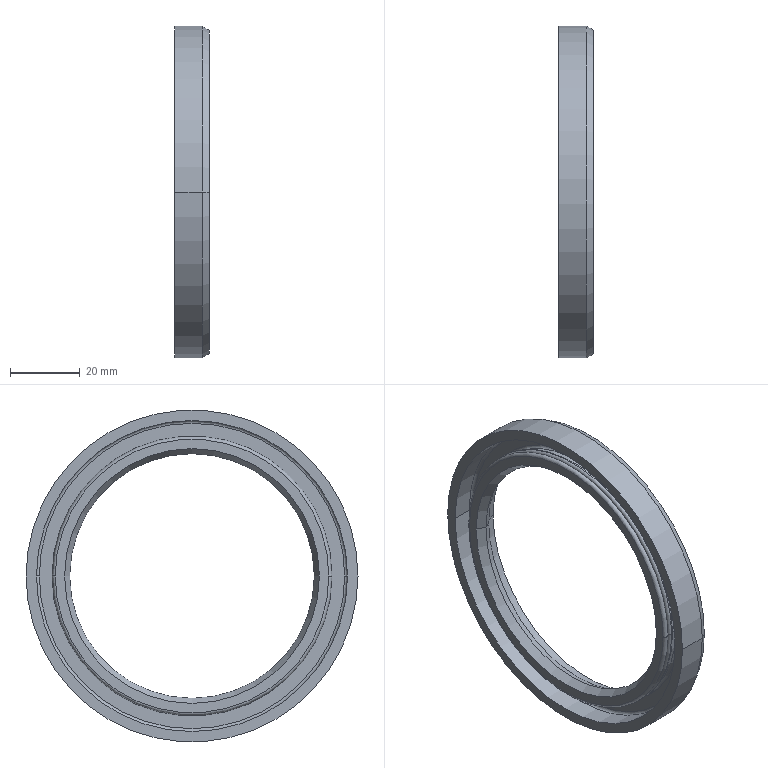Part | SolidWorks | features Revolution 1 | 2 solids | 58 faces | box 10 x 95 x 95 mm | volume 15410 mm3 | torus 22 | cylinder 16 | cone 10 | plane 10 | commonest cylinder face diameters 78.5 x2 82 x2 82.5 x2 86 x2 89 x2 91 x2
STEP:
#1=CARTESIAN_POINT('',(-7.9,-39.15,0.));
#2=VERTEX_POINT('',#1);
#3=CARTESIAN_POINT('',(-6.9,-38.199,0.));
#4=VERTEX_POINT('',#3);
#5=CARTESIAN_POINT('',(-6.9,-39.2,0.));
#6=DIRECTION('',(0.,0.,-1.));
#7=DIRECTION('',(-1.,0.,0.));
#8=AXIS2_PLACEMENT_3D('',#5,#6,#7);
#9=CIRCLE('',#8,1.001);
#10=EDGE_CURVE('',#2,#4,#9,.T.);
#11=ORIENTED_EDGE('',*,*,#10,.T.);
#12=CARTESIAN_POINT('',(-6.9,38.199,0.));
#13=VERTEX_POINT('',#12);
#14=CARTESIAN_POINT('',(-6.9,0.,0.));
#15=DIRECTION('',(-1.,0.,0.));
#16=DIRECTION('',(0.,-1.,0.));
#17=AXIS2_PLACEMENT_3D('',#14,#15,#16);
#18=CIRCLE('',#17,38.199);
#19=EDGE_CURVE('',#4,#13,#18,.T.);
#20=ORIENTED_EDGE('',*,*,#19,.T.);
#21=CARTESIAN_POINT('',(-7.9,39.15,0.));
#22=VERTEX_POINT('',#21);
#23=CARTESIAN_POINT('',(-6.9,39.2,0.));
#24=DIRECTION('',(0.,0.,1.));
#25=DIRECTION('',(0.,-1.,0.));
#26=AXIS2_PLACEMENT_3D('',#23,#24,#25);
#27=CIRCLE('',#26,1.001);
#28=EDGE_CURVE('',#22,#13,#27,.T.);
#29=ORIENTED_EDGE('',*,*,#28,.F.);
#30=CARTESIAN_POINT('',(-7.9,0.,0.));
#31=DIRECTION('',(-1.,0.,0.));
#32=DIRECTION('',(0.,-1.,0.));
#33=AXIS2_PLACEMENT_3D('',#30,#31,#32);
#34=CIRCLE('',#33,39.15);
#35=EDGE_CURVE('',#2,#22,#34,.T.);
#36=ORIENTED_EDGE('',*,*,#35,.F.);
#37=EDGE_LOOP('',(#11,#20,#29,#36));
#38=FACE_OUTER_BOUND('',#37,.T.);
#39=CARTESIAN_POINT('',(-6.9,0.,0.));
#40=DIRECTION('',(-1.,0.,0.));
#41=DIRECTION('',(0.,-1.,0.));
#42=AXIS2_PLACEMENT_3D('',#39,#40,#41);
#43=TOROIDAL_SURFACE('',#42,39.2,1.001);
#44=ADVANCED_FACE('',(#38),#43,.F.);
#45=ORIENTED_EDGE('',*,*,#28,.T.);
#46=CARTESIAN_POINT('',(-6.9,0.,0.));
#47=DIRECTION('',(-1.,0.,0.));
#48=DIRECTION('',(0.,-1.,0.));
#49=AXIS2_PLACEMENT_3D('',#46,#47,#48);
#50=CIRCLE('',#49,38.199);
#51=EDGE_CURVE('',#13,#4,#50,.T.);
#52=ORIENTED_EDGE('',*,*,#51,.T.);
#53=ORIENTED_EDGE('',*,*,#10,.F.);
#54=CARTESIAN_POINT('',(-7.9,0.,0.));
#55=DIRECTION('',(-1.,0.,0.));
#56=DIRECTION('',(0.,-1.,0.));
#57=AXIS2_PLACEMENT_3D('',#54,#55,#56);
#58=CIRCLE('',#57,39.15);
#59=EDGE_CURVE('',#22,#2,#58,.T.);
#60=ORIENTED_EDGE('',*,*,#59,.F.);
#61=EDGE_LOOP('',(#45,#52,#53,#60));
#62=FACE_OUTER_BOUND('',#61,.T.);
#63=CARTESIAN_POINT('',(-6.9,0.,0.));
#64=DIRECTION('',(-1.,0.,0.));
#65=DIRECTION('',(0.,-1.,0.));
#66=AXIS2_PLACEMENT_3D('',#63,#64,#65);
#67=TOROIDAL_SURFACE('',#66,39.2,1.001);
#68=ADVANCED_FACE('',(#62),#67,.F.);
#69=CARTESIAN_POINT('',(-4.3,-39.25,0.));
#70=VERTEX_POINT('',#69);
#71=CARTESIAN_POINT('',(-4.3,39.25,0.));
#72=VERTEX_POINT('',#71);
#73=CARTESIAN_POINT('',(-4.3,0.,0.));
#74=DIRECTION('',(-1.,0.,0.));
#75=DIRECTION('',(0.,-1.,0.));
#76=AXIS2_PLACEMENT_3D('',#73,#74,#75);
#77=CIRCLE('',#76,39.25);
#78=EDGE_CURVE('',#70,#72,#77,.T.);
#79=ORIENTED_EDGE('',*,*,#78,.T.);
#80=CARTESIAN_POINT('',(-5.9,39.25,0.));
#81=VERTEX_POINT('',#80);
#82=CARTESIAN_POINT('',(-10.,39.25,0.));
#83=DIRECTION('',(-1.,0.,0.));
#84=VECTOR('',#83,1000.);
#85=LINE('',#82,#84);
#86=EDGE_CURVE('',#72,#81,#85,.T.);
#87=ORIENTED_EDGE('',*,*,#86,.T.);
#88=CARTESIAN_POINT('',(-5.9,-39.25,0.));
#89=VERTEX_POINT('',#88);
#90=CARTESIAN_POINT('',(-5.9,0.,0.));
#91=DIRECTION('',(-1.,0.,0.));
#92=DIRECTION('',(0.,-1.,0.));
#93=AXIS2_PLACEMENT_3D('',#90,#91,#92);
#94=CIRCLE('',#93,39.25);
#95=EDGE_CURVE('',#89,#81,#94,.T.);
#96=ORIENTED_EDGE('',*,*,#95,.F.);
#97=CARTESIAN_POINT('',(-10.,-39.25,0.));
#98=DIRECTION('',(-1.,0.,0.));
#99=VECTOR('',#98,1000.);
#100=LINE('',#97,#99);
#101=EDGE_CURVE('',#70,#89,#100,.T.);
#102=ORIENTED_EDGE('',*,*,#101,.F.);
#103=EDGE_LOOP('',(#79,#87,#96,#102));
#104=FACE_OUTER_BOUND('',#103,.T.);
#105=CARTESIAN_POINT('',(-10.,0.,0.));
#106=DIRECTION('',(-1.,0.,0.));
#107=DIRECTION('',(0.,-1.,0.));
#108=AXIS2_PLACEMENT_3D('',#105,#106,#107);
#109=CYLINDRICAL_SURFACE('',#108,39.25);
#110=ADVANCED_FACE('',(#104),#109,.T.);
#111=CARTESIAN_POINT('',(-4.3,0.,0.));
#112=DIRECTION('',(-1.,0.,0.));
#113=DIRECTION('',(0.,-1.,0.));
#114=AXIS2_PLACEMENT_3D('',#111,#112,#113);
#115=CIRCLE('',#114,39.25);
#116=EDGE_CURVE('',#72,#70,#115,.T.);
#117=ORIENTED_EDGE('',*,*,#116,.F.);
#118=CARTESIAN_POINT('',(-3.5,40.05,0.));
#119=VERTEX_POINT('',#118);
#120=CARTESIAN_POINT('',(-4.3,40.05,0.));
#121=DIRECTION('',(0.,0.,1.));
#122=DIRECTION('',(0.,-1.,0.));
#123=AXIS2_PLACEMENT_3D('',#120,#121,#122);
#124=CIRCLE('',#123,0.8);
#125=EDGE_CURVE('',#72,#119,#124,.T.);
#126=ORIENTED_EDGE('',*,*,#125,.T.);
#127=CARTESIAN_POINT('',(-3.5,-40.05,0.));
#128=VERTEX_POINT('',#127);
#129=CARTESIAN_POINT('',(-3.5,0.,0.));
#130=DIRECTION('',(-1.,0.,0.));
#131=DIRECTION('',(0.,-1.,0.));
#132=AXIS2_PLACEMENT_3D('',#129,#130,#131);
#133=CIRCLE('',#132,40.05);
#134=EDGE_CURVE('',#119,#128,#133,.T.);
#135=ORIENTED_EDGE('',*,*,#134,.T.);
#136=CARTESIAN_POINT('',(-4.3,-40.05,0.));
#137=DIRECTION('',(0.,0.,-1.));
#138=DIRECTION('',(-1.,0.,0.));
#139=AXIS2_PLACEMENT_3D('',#136,#137,#138);
#140=CIRCLE('',#139,0.8);
#141=EDGE_CURVE('',#70,#128,#140,.T.);
#142=ORIENTED_EDGE('',*,*,#141,.F.);
#143=EDGE_LOOP('',(#117,#126,#135,#142));
#144=FACE_OUTER_BOUND('',#143,.T.);
#145=CARTESIAN_POINT('',(-4.3,0.,0.));
#146=DIRECTION('',(-1.,0.,0.));
#147=DIRECTION('',(0.,-1.,0.));
#148=AXIS2_PLACEMENT_3D('',#145,#146,#147);
#149=TOROIDAL_SURFACE('',#148,40.05,0.8);
#150=ADVANCED_FACE('',(#144),#149,.F.);
#151=CARTESIAN_POINT('',(-3.5,43.7,0.));
#152=VERTEX_POINT('',#151);
#153=CARTESIAN_POINT('',(-3.5,-43.7,0.));
#154=VERTEX_POINT('',#153);
#155=CARTESIAN_POINT('',(-3.5,0.,0.));
#156=DIRECTION('',(-1.,0.,0.));
#157=DIRECTION('',(0.,-1.,0.));
#158=AXIS2_PLACEMENT_3D('',#155,#156,#157);
#159=CIRCLE('',#158,43.7);
#160=EDGE_CURVE('',#152,#154,#159,.T.);
#161=ORIENTED_EDGE('',*,*,#160,.F.);
#162=CARTESIAN_POINT('',(-4.3,44.5,0.));
#163=VERTEX_POINT('',#162);
#164=CARTESIAN_POINT('',(-4.3,43.7,0.));
#165=DIRECTION('',(0.,0.,1.));
#166=DIRECTION('',(0.,-1.,0.));
#167=AXIS2_PLACEMENT_3D('',#164,#165,#166);
#168=CIRCLE('',#167,0.8);
#169=EDGE_CURVE('',#152,#163,#168,.T.);
#170=ORIENTED_EDGE('',*,*,#169,.T.);
#171=CARTESIAN_POINT('',(-4.3,-44.5,0.));
#172=VERTEX_POINT('',#171);
#173=CARTESIAN_POINT('',(-4.3,0.,0.));
#174=DIRECTION('',(-1.,0.,0.));
#175=DIRECTION('',(0.,-1.,0.));
#176=AXIS2_PLACEMENT_3D('',#173,#174,#175);
#177=CIRCLE('',#176,44.5);
#178=EDGE_CURVE('',#163,#172,#177,.T.);
#179=ORIENTED_EDGE('',*,*,#178,.T.);
#180=CARTESIAN_POINT('',(-4.3,-43.7,0.));
#181=DIRECTION('',(0.,0.,-1.));
#182=DIRECTION('',(-1.,0.,0.));
#183=AXIS2_PLACEMENT_3D('',#180,#181,#182);
#184=CIRCLE('',#183,0.8);
#185=EDGE_CURVE('',#154,#172,#184,.T.);
#186=ORIENTED_EDGE('',*,*,#185,.F.);
#187=EDGE_LOOP('',(#161,#170,#179,#186));
#188=FACE_OUTER_BOUND('',#187,.T.);
#189=CARTESIAN_POINT('',(-4.3,0.,0.));
#190=DIRECTION('',(-1.,0.,0.));
#191=DIRECTION('',(0.,-1.,0.));
#192=AXIS2_PLACEMENT_3D('',#189,#190,#191);
#193=TOROIDAL_SURFACE('',#192,43.7,0.8);
#194=ADVANCED_FACE('',(#188),#193,.F.);
#195=ORIENTED_EDGE('',*,*,#178,.F.);
#196=CARTESIAN_POINT('',(-10.,44.5,0.));
#197=VERTEX_POINT('',#196);
#198=CARTESIAN_POINT('',(-10.,44.5,0.));
#199=DIRECTION('',(-1.,0.,0.));
#200=VECTOR('',#199,1000.);
#201=LINE('',#198,#200);
#202=EDGE_CURVE('',#163,#197,#201,.T.);
#203=ORIENTED_EDGE('',*,*,#202,.T.);
#204=CARTESIAN_POINT('',(-10.,-44.5,0.));
#205=VERTEX_POINT('',#204);
#206=CARTESIAN_POINT('',(-10.,0.,0.));
#207=DIRECTION('',(-1.,0.,0.));
#208=DIRECTION('',(0.,-1.,0.));
#209=AXIS2_PLACEMENT_3D('',#206,#207,#208);
#210=CIRCLE('',#209,44.5);
#211=EDGE_CURVE('',#197,#205,#210,.T.);
#212=ORIENTED_EDGE('',*,*,#211,.T.);
#213=CARTESIAN_POINT('',(-10.,-44.5,0.));
#214=DIRECTION('',(-1.,0.,0.));
#215=VECTOR('',#214,1000.);
#216=LINE('',#213,#215);
#217=EDGE_CURVE('',#172,#205,#216,.T.);
#218=ORIENTED_EDGE('',*,*,#217,.F.);
#219=EDGE_LOOP('',(#195,#203,#212,#218));
#220=FACE_OUTER_BOUND('',#219,.T.);
#221=CARTESIAN_POINT('',(-10.,0.,0.));
#222=DIRECTION('',(-1.,0.,0.));
#223=DIRECTION('',(0.,-1.,0.));
#224=AXIS2_PLACEMENT_3D('',#221,#222,#223);
#225=CYLINDRICAL_SURFACE('',#224,44.5);
#226=ADVANCED_FACE('',(#220),#225,.F.);
#227=CARTESIAN_POINT('',(-2.,-47.5,0.));
#228=VERTEX_POINT('',#227);
#229=CARTESIAN_POINT('',(-2.,47.5,0.));
#230=VERTEX_POINT('',#229);
#231=CARTESIAN_POINT('',(-2.,0.,0.));
#232=DIRECTION('',(-1.,0.,0.));
#233=DIRECTION('',(0.,-1.,0.));
#234=AXIS2_PLACEMENT_3D('',#231,#232,#233);
#235=CIRCLE('',#234,47.5);
#236=EDGE_CURVE('',#228,#230,#235,.T.);
#237=ORIENTED_EDGE('',*,*,#236,.T.);
#238=CARTESIAN_POINT('',(-10.,47.5,0.));
#239=VERTEX_POINT('',#238);
#240=CARTESIAN_POINT('',(-10.,47.5,0.));
#241=DIRECTION('',(-1.,0.,0.));
#242=VECTOR('',#241,1000.);
#243=LINE('',#240,#242);
#244=EDGE_CURVE('',#230,#239,#243,.T.);
#245=ORIENTED_EDGE('',*,*,#244,.T.);
#246=CARTESIAN_POINT('',(-10.,-47.5,0.));
#247=VERTEX_POINT('',#246);
#248=CARTESIAN_POINT('',(-10.,0.,0.));
#249=DIRECTION('',(-1.,0.,0.));
#250=DIRECTION('',(0.,-1.,0.));
#251=AXIS2_PLACEMENT_3D('',#248,#249,#250);
#252=CIRCLE('',#251,47.5);
#253=EDGE_CURVE('',#247,#239,#252,.T.);
#254=ORIENTED_EDGE('',*,*,#253,.F.);
#255=CARTESIAN_POINT('',(-10.,-47.5,0.));
#256=DIRECTION('',(-1.,0.,0.));
#257=VECTOR('',#256,1000.);
#258=LINE('',#255,#257);
#259=EDGE_CURVE('',#228,#247,#258,.T.);
#260=ORIENTED_EDGE('',*,*,#259,.F.);
#261=EDGE_LOOP('',(#237,#245,#254,#260));
#262=FACE_OUTER_BOUND('',#261,.T.);
#263=CARTESIAN_POINT('',(-10.,0.,0.));
#264=DIRECTION('',(-1.,0.,0.));
#265=DIRECTION('',(0.,-1.,0.));
#266=AXIS2_PLACEMENT_3D('',#263,#264,#265);
#267=CYLINDRICAL_SURFACE('',#266,47.5);
#268=ADVANCED_FACE('',(#262),#267,.T.);
#269=CARTESIAN_POINT('',(0.,-46.345,0.));
#270=VERTEX_POINT('',#269);
#271=CARTESIAN_POINT('',(0.,46.345,0.));
#272=VERTEX_POINT('',#271);
#273=CARTESIAN_POINT('',(0.,0.,0.));
#274=DIRECTION('',(-1.,0.,0.));
#275=DIRECTION('',(0.,-1.,0.));
#276=AXIS2_PLACEMENT_3D('',#273,#274,#275);
#277=CIRCLE('',#276,46.345);
#278=EDGE_CURVE('',#270,#272,#277,.T.);
#279=ORIENTED_EDGE('',*,*,#278,.T.);
#280=CARTESIAN_POINT('',(-2.,47.5,0.));
#281=DIRECTION('',(-0.866,0.5,0.));
#282=VECTOR('',#281,1000.);
#283=LINE('',#280,#282);
#284=EDGE_CURVE('',#272,#230,#283,.T.);
#285=ORIENTED_EDGE('',*,*,#284,.T.);
#286=ORIENTED_EDGE('',*,*,#236,.F.);
#287=CARTESIAN_POINT('',(-2.,-47.5,0.));
#288=DIRECTION('',(-0.866,-0.5,0.));
#289=VECTOR('',#288,1000.);
#290=LINE('',#287,#289);
#291=EDGE_CURVE('',#270,#228,#290,.T.);
#292=ORIENTED_EDGE('',*,*,#291,.F.);
#293=EDGE_LOOP('',(#279,#285,#286,#292));
#294=FACE_OUTER_BOUND('',#293,.T.);
#295=CARTESIAN_POINT('',(-2.,0.,0.));
#296=DIRECTION('',(-1.,0.,0.));
#297=DIRECTION('',(0.,-1.,0.));
#298=AXIS2_PLACEMENT_3D('',#295,#296,#297);
#299=CONICAL_SURFACE('',#298,47.5,0.5236);
#300=ADVANCED_FACE('',(#294),#299,.T.);
#301=CARTESIAN_POINT('',(0.,43.,0.));
#302=VERTEX_POINT('',#301);
#303=CARTESIAN_POINT('',(0.,-43.,0.));
#304=VERTEX_POINT('',#303);
#305=CARTESIAN_POINT('',(0.,0.,0.));
#306=DIRECTION('',(-1.,0.,0.));
#307=DIRECTION('',(0.,-1.,0.));
#308=AXIS2_PLACEMENT_3D('',#305,#306,#307);
#309=CIRCLE('',#308,43.);
#310=EDGE_CURVE('',#302,#304,#309,.T.);
#311=ORIENTED_EDGE('',*,*,#310,.F.);
#312=CARTESIAN_POINT('',(-1.,43.,0.));
#313=VERTEX_POINT('',#312);
#314=CARTESIAN_POINT('',(-10.,43.,0.));
#315=DIRECTION('',(-1.,0.,0.));
#316=VECTOR('',#315,1000.);
#317=LINE('',#314,#316);
#318=EDGE_CURVE('',#302,#313,#317,.T.);
#319=ORIENTED_EDGE('',*,*,#318,.T.);
#320=CARTESIAN_POINT('',(-1.,-43.,0.));
#321=VERTEX_POINT('',#320);
#322=CARTESIAN_POINT('',(-1.,0.,0.));
#323=DIRECTION('',(-1.,0.,0.));
#324=DIRECTION('',(0.,-1.,0.));
#325=AXIS2_PLACEMENT_3D('',#322,#323,#324);
#326=CIRCLE('',#325,43.);
#327=EDGE_CURVE('',#313,#321,#326,.T.);
#328=ORIENTED_EDGE('',*,*,#327,.T.);
#329=CARTESIAN_POINT('',(-10.,-43.,0.));
#330=DIRECTION('',(-1.,0.,0.));
#331=VECTOR('',#330,1000.);
#332=LINE('',#329,#331);
#333=EDGE_CURVE('',#304,#321,#332,.T.);
#334=ORIENTED_EDGE('',*,*,#333,.F.);
#335=EDGE_LOOP('',(#311,#319,#328,#334));
#336=FACE_OUTER_BOUND('',#335,.T.);
#337=CARTESIAN_POINT('',(-10.,0.,0.));
#338=DIRECTION('',(-1.,0.,0.));
#339=DIRECTION('',(0.,-1.,0.));
#340=AXIS2_PLACEMENT_3D('',#337,#338,#339);
#341=CYLINDRICAL_SURFACE('',#340,43.);
#342=ADVANCED_FACE('',(#336),#341,.F.);
#343=CARTESIAN_POINT('',(0.,-41.,0.));
#344=VERTEX_POINT('',#343);
#345=CARTESIAN_POINT('',(0.,41.,0.));
#346=VERTEX_POINT('',#345);
#347=CARTESIAN_POINT('',(0.,0.,0.));
#348=DIRECTION('',(-1.,0.,0.));
#349=DIRECTION('',(0.,-1.,0.));
#350=AXIS2_PLACEMENT_3D('',#347,#348,#349);
#351=CIRCLE('',#350,41.);
#352=EDGE_CURVE('',#344,#346,#351,.T.);
#353=ORIENTED_EDGE('',*,*,#352,.T.);
#354=CARTESIAN_POINT('',(-1.,41.,0.));
#355=VERTEX_POINT('',#354);
#356=CARTESIAN_POINT('',(-10.,41.,0.));
#357=DIRECTION('',(-1.,0.,0.));
#358=VECTOR('',#357,1000.);
#359=LINE('',#356,#358);
#360=EDGE_CURVE('',#346,#355,#359,.T.);
#361=ORIENTED_EDGE('',*,*,#360,.T.);
#362=CARTESIAN_POINT('',(-1.,-41.,0.));
#363=VERTEX_POINT('',#362);
#364=CARTESIAN_POINT('',(-1.,0.,0.));
#365=DIRECTION('',(-1.,0.,0.));
#366=DIRECTION('',(0.,-1.,0.));
#367=AXIS2_PLACEMENT_3D('',#364,#365,#366);
#368=CIRCLE('',#367,41.);
#369=EDGE_CURVE('',#363,#355,#368,.T.);
#370=ORIENTED_EDGE('',*,*,#369,.F.);
#371=CARTESIAN_POINT('',(-10.,-41.,0.));
#372=DIRECTION('',(-1.,0.,0.));
#373=VECTOR('',#372,1000.);
#374=LINE('',#371,#373);
#375=EDGE_CURVE('',#344,#363,#374,.T.);
#376=ORIENTED_EDGE('',*,*,#375,.F.);
#377=EDGE_LOOP('',(#353,#361,#370,#376));
#378=FACE_OUTER_BOUND('',#377,.T.);
#379=CARTESIAN_POINT('',(-10.,0.,0.));
#380=DIRECTION('',(-1.,0.,0.));
#381=DIRECTION('',(0.,-1.,0.));
#382=AXIS2_PLACEMENT_3D('',#379,#380,#381);
#383=CYLINDRICAL_SURFACE('',#382,41.);
#384=ADVANCED_FACE('',(#378),#383,.T.);
#385=CARTESIAN_POINT('',(-1.155,38.,0.));
#386=VERTEX_POINT('',#385);
#387=CARTESIAN_POINT('',(-1.155,-38.,0.));
#388=VERTEX_POINT('',#387);
#389=CARTESIAN_POINT('',(-1.155,0.,0.));
#390=DIRECTION('',(-1.,0.,0.));
#391=DIRECTION('',(0.,-1.,0.));
#392=AXIS2_PLACEMENT_3D('',#389,#390,#391);
#393=CIRCLE('',#392,38.);
#394=EDGE_CURVE('',#386,#388,#393,.T.);
#395=ORIENTED_EDGE('',*,*,#394,.T.);
#396=CARTESIAN_POINT('',(0.,-40.,0.));
#397=VERTEX_POINT('',#396);
#398=CARTESIAN_POINT('',(-1.155,-38.,0.));
#399=DIRECTION('',(0.5,-0.866,0.));
#400=VECTOR('',#399,1000.);
#401=LINE('',#398,#400);
#402=EDGE_CURVE('',#388,#397,#401,.T.);
#403=ORIENTED_EDGE('',*,*,#402,.T.);
#404=CARTESIAN_POINT('',(0.,40.,0.));
#405=VERTEX_POINT('',#404);
#406=CARTESIAN_POINT('',(0.,0.,0.));
#407=DIRECTION('',(-1.,0.,0.));
#408=DIRECTION('',(0.,-1.,0.));
#409=AXIS2_PLACEMENT_3D('',#406,#407,#408);
#410=CIRCLE('',#409,40.);
#411=EDGE_CURVE('',#405,#397,#410,.T.);
#412=ORIENTED_EDGE('',*,*,#411,.F.);
#413=CARTESIAN_POINT('',(-1.155,38.,0.));
#414=DIRECTION('',(0.5,0.866,0.));
#415=VECTOR('',#414,1000.);
#416=LINE('',#413,#415);
#417=EDGE_CURVE('',#386,#405,#416,.T.);
#418=ORIENTED_EDGE('',*,*,#417,.F.);
#419=EDGE_LOOP('',(#395,#403,#412,#418));
#420=FACE_OUTER_BOUND('',#419,.T.);
#421=CARTESIAN_POINT('',(-1.155,0.,0.));
#422=DIRECTION('',(1.,0.,0.));
#423=DIRECTION('',(0.,1.,0.));
#424=AXIS2_PLACEMENT_3D('',#421,#422,#423);
#425=CONICAL_SURFACE('',#424,38.,1.047);
#426=ADVANCED_FACE('',(#420),#425,.F.);
#427=CARTESIAN_POINT('',(-4.5,36.943,0.));
#428=VERTEX_POINT('',#427);
#429=CARTESIAN_POINT('',(-4.5,-36.943,0.));
#430=VERTEX_POINT('',#429);
#431=CARTESIAN_POINT('',(-4.5,0.,0.));
#432=DIRECTION('',(-1.,0.,0.));
#433=DIRECTION('',(0.,-1.,0.));
#434=AXIS2_PLACEMENT_3D('',#431,#432,#433);
#435=CIRCLE('',#434,36.943);
#436=EDGE_CURVE('',#428,#430,#435,.T.);
#437=ORIENTED_EDGE('',*,*,#436,.T.);
#438=CARTESIAN_POINT('',(-4.5,-36.943,0.));
#439=DIRECTION('',(0.9536,-0.3012,0.));
#440=VECTOR('',#439,1000.);
#441=LINE('',#438,#440);
#442=EDGE_CURVE('',#430,#388,#441,.T.);
#443=ORIENTED_EDGE('',*,*,#442,.T.);
#444=ORIENTED_EDGE('',*,*,#394,.F.);
#445=CARTESIAN_POINT('',(-4.5,36.943,0.));
#446=DIRECTION('',(0.9536,0.3012,0.));
#447=VECTOR('',#446,1000.);
#448=LINE('',#445,#447);
#449=EDGE_CURVE('',#428,#386,#448,.T.);
#450=ORIENTED_EDGE('',*,*,#449,.F.);
#451=EDGE_LOOP('',(#437,#443,#444,#450));
#452=FACE_OUTER_BOUND('',#451,.T.);
#453=CARTESIAN_POINT('',(-4.5,0.,0.));
#454=DIRECTION('',(1.,0.,0.));
#455=DIRECTION('',(0.,1.,0.));
#456=AXIS2_PLACEMENT_3D('',#453,#454,#455);
#457=CONICAL_SURFACE('',#456,36.943,0.3059);
#458=ADVANCED_FACE('',(#452),#457,.F.);
#459=CARTESIAN_POINT('',(-7.,35.,0.));
#460=VERTEX_POINT('',#459);
#461=CARTESIAN_POINT('',(-7.,-35.,0.));
#462=VERTEX_POINT('',#461);
#463=CARTESIAN_POINT('',(-7.,0.,0.));
#464=DIRECTION('',(-1.,0.,0.));
#465=DIRECTION('',(0.,-1.,0.));
#466=AXIS2_PLACEMENT_3D('',#463,#464,#465);
#467=CIRCLE('',#466,35.);
#468=EDGE_CURVE('',#460,#462,#467,.T.);
#469=ORIENTED_EDGE('',*,*,#468,.T.);
#470=CARTESIAN_POINT('',(-4.5,-36.443,0.));
#471=VERTEX_POINT('',#470);
#472=CARTESIAN_POINT('',(-7.,-35.,0.));
#473=DIRECTION('',(0.866,-0.5,0.));
#474=VECTOR('',#473,1000.);
#475=LINE('',#472,#474);
#476=EDGE_CURVE('',#462,#471,#475,.T.);
#477=ORIENTED_EDGE('',*,*,#476,.T.);
#478=CARTESIAN_POINT('',(-4.5,36.443,0.));
#479=VERTEX_POINT('',#478);
#480=CARTESIAN_POINT('',(-4.5,0.,0.));
#481=DIRECTION('',(-1.,0.,0.));
#482=DIRECTION('',(0.,-1.,0.));
#483=AXIS2_PLACEMENT_3D('',#480,#481,#482);
#484=CIRCLE('',#483,36.443);
#485=EDGE_CURVE('',#479,#471,#484,.T.);
#486=ORIENTED_EDGE('',*,*,#485,.F.);
#487=CARTESIAN_POINT('',(-7.,35.,0.));
#488=DIRECTION('',(0.866,0.5,0.));
#489=VECTOR('',#488,1000.);
#490=LINE('',#487,#489);
#491=EDGE_CURVE('',#460,#479,#490,.T.);
#492=ORIENTED_EDGE('',*,*,#491,.F.);
#493=EDGE_LOOP('',(#469,#477,#486,#492));
#494=FACE_OUTER_BOUND('',#493,.T.);
#495=CARTESIAN_POINT('',(-7.,0.,0.));
#496=DIRECTION('',(1.,0.,0.));
#497=DIRECTION('',(0.,1.,0.));
#498=AXIS2_PLACEMENT_3D('',#495,#496,#497);
#499=CONICAL_SURFACE('',#498,35.,0.5236);
#500=ADVANCED_FACE('',(#494),#499,.F.);
#501=ORIENTED_EDGE('',*,*,#468,.F.);
#502=CARTESIAN_POINT('',(-9.5,36.443,0.));
#503=VERTEX_POINT('',#502);
#504=CARTESIAN_POINT('',(-9.5,36.443,0.));
#505=DIRECTION('',(-0.866,0.5,0.));
#506=VECTOR('',#505,1000.);
#507=LINE('',#504,#506);
#508=EDGE_CURVE('',#460,#503,#507,.T.);
#509=ORIENTED_EDGE('',*,*,#508,.T.);
#510=CARTESIAN_POINT('',(-9.5,-36.443,0.));
#511=VERTEX_POINT('',#510);
#512=CARTESIAN_POINT('',(-9.5,0.,0.));
#513=DIRECTION('',(-1.,0.,0.));
#514=DIRECTION('',(0.,-1.,0.));
#515=AXIS2_PLACEMENT_3D('',#512,#513,#514);
#516=CIRCLE('',#515,36.443);
#517=EDGE_CURVE('',#503,#511,#516,.T.);
#518=ORIENTED_EDGE('',*,*,#517,.T.);
#519=CARTESIAN_POINT('',(-9.5,-36.443,0.));
#520=DIRECTION('',(-0.866,-0.5,0.));
#521=VECTOR('',#520,1000.);
#522=LINE('',#519,#521);
#523=EDGE_CURVE('',#462,#511,#522,.T.);
#524=ORIENTED_EDGE('',*,*,#523,.F.);
#525=EDGE_LOOP('',(#501,#509,#518,#524));
#526=FACE_OUTER_BOUND('',#525,.T.);
#527=CARTESIAN_POINT('',(-9.5,0.,0.));
#528=DIRECTION('',(-1.,0.,0.));
#529=DIRECTION('',(0.,-1.,0.));
#530=AXIS2_PLACEMENT_3D('',#527,#528,#529);
#531=CONICAL_SURFACE('',#530,36.443,0.5236);
#532=ADVANCED_FACE('',(#526),#531,.F.);
#533=ORIENTED_EDGE('',*,*,#35,.T.);
#534=CARTESIAN_POINT('',(-9.5,39.15,0.));
#535=VERTEX_POINT('',#534);
#536=CARTESIAN_POINT('',(-8.7,39.15,0.));
#537=DIRECTION('',(0.,0.,1.));
#538=DIRECTION('',(0.,-1.,0.));
#539=AXIS2_PLACEMENT_3D('',#536,#537,#538);
#540=CIRCLE('',#539,0.8);
#541=EDGE_CURVE('',#22,#535,#540,.T.);
#542=ORIENTED_EDGE('',*,*,#541,.T.);
#543=CARTESIAN_POINT('',(-9.5,-39.15,0.));
#544=VERTEX_POINT('',#543);
#545=CARTESIAN_POINT('',(-9.5,0.,0.));
#546=DIRECTION('',(-1.,0.,0.));
#547=DIRECTION('',(0.,-1.,0.));
#548=AXIS2_PLACEMENT_3D('',#545,#546,#547);
#549=CIRCLE('',#548,39.15);
#550=EDGE_CURVE('',#544,#535,#549,.T.);
#551=ORIENTED_EDGE('',*,*,#550,.F.);
#552=CARTESIAN_POINT('',(-8.7,-39.15,0.));
#553=DIRECTION('',(0.,0.,-1.));
#554=DIRECTION('',(-1.,0.,0.));
#555=AXIS2_PLACEMENT_3D('',#552,#553,#554);
#556=CIRCLE('',#555,0.8);
#557=EDGE_CURVE('',#2,#544,#556,.T.);
#558=ORIENTED_EDGE('',*,*,#557,.F.);
#559=EDGE_LOOP('',(#533,#542,#551,#558));
#560=FACE_OUTER_BOUND('',#559,.T.);
#561=CARTESIAN_POINT('',(-8.7,0.,0.));
#562=DIRECTION('',(-1.,0.,0.));
#563=DIRECTION('',(0.,-1.,0.));
#564=AXIS2_PLACEMENT_3D('',#561,#562,#563);
#565=TOROIDAL_SURFACE('',#564,39.15,0.8);
#566=ADVANCED_FACE('',(#560),#565,.T.);
#567=ORIENTED_EDGE('',*,*,#51,.F.);
#568=CARTESIAN_POINT('',(-6.9,39.2,0.));
#569=DIRECTION('',(0.,0.,1.));
#570=DIRECTION('',(0.,-1.,0.));
#571=AXIS2_PLACEMENT_3D('',#568,#569,#570);
#572=CIRCLE('',#571,1.001);
#573=EDGE_CURVE('',#13,#81,#572,.T.);
#574=ORIENTED_EDGE('',*,*,#573,.T.);
#575=CARTESIAN_POINT('',(-5.9,0.,0.));
#576=DIRECTION('',(-1.,0.,0.));
#577=DIRECTION('',(0.,-1.,0.));
#578=AXIS2_PLACEMENT_3D('',#575,#576,#577);
#579=CIRCLE('',#578,39.25);
#580=EDGE_CURVE('',#81,#89,#579,.T.);
#581=ORIENTED_EDGE('',*,*,#580,.T.);
#582=CARTESIAN_POINT('',(-6.9,-39.2,0.));
#583=DIRECTION('',(0.,0.,-1.));
#584=DIRECTION('',(-1.,0.,0.));
#585=AXIS2_PLACEMENT_3D('',#582,#583,#584);
#586=CIRCLE('',#585,1.001);
#587=EDGE_CURVE('',#4,#89,#586,.T.);
#588=ORIENTED_EDGE('',*,*,#587,.F.);
#589=EDGE_LOOP('',(#567,#574,#581,#588));
#590=FACE_OUTER_BOUND('',#589,.T.);
#591=CARTESIAN_POINT('',(-6.9,0.,0.));
#592=DIRECTION('',(-1.,0.,0.));
#593=DIRECTION('',(0.,-1.,0.));
#594=AXIS2_PLACEMENT_3D('',#591,#592,#593);
#595=TOROIDAL_SURFACE('',#594,39.2,1.001);
#596=ADVANCED_FACE('',(#590),#595,.F.);
#597=ORIENTED_EDGE('',*,*,#19,.F.);
#598=ORIENTED_EDGE('',*,*,#587,.T.);
#599=ORIENTED_EDGE('',*,*,#95,.T.);
#600=ORIENTED_EDGE('',*,*,#573,.F.);
#601=EDGE_LOOP('',(#597,#598,#599,#600));
#602=FACE_OUTER_BOUND('',#601,.T.);
#603=CARTESIAN_POINT('',(-6.9,0.,0.));
#604=DIRECTION('',(-1.,0.,0.));
#605=DIRECTION('',(0.,-1.,0.));
#606=AXIS2_PLACEMENT_3D('',#603,#604,#605);
#607=TOROIDAL_SURFACE('',#606,39.2,1.001);
#608=ADVANCED_FACE('',(#602),#607,.F.);
#609=ORIENTED_EDGE('',*,*,#541,.F.);
#610=ORIENTED_EDGE('',*,*,#59,.T.);
#611=ORIENTED_EDGE('',*,*,#557,.T.);
#612=CARTESIAN_POINT('',(-9.5,0.,0.));
#613=DIRECTION('',(-1.,0.,0.));
#614=DIRECTION('',(0.,-1.,0.));
#615=AXIS2_PLACEMENT_3D('',#612,#613,#614);
#616=CIRCLE('',#615,39.15);
#617=EDGE_CURVE('',#535,#544,#616,.T.);
#618=ORIENTED_EDGE('',*,*,#617,.F.);
#619=EDGE_LOOP('',(#609,#610,#611,#618));
#620=FACE_OUTER_BOUND('',#619,.T.);
#621=CARTESIAN_POINT('',(-8.7,0.,0.));
#622=DIRECTION('',(-1.,0.,0.));
#623=DIRECTION('',(0.,-1.,0.));
#624=AXIS2_PLACEMENT_3D('',#621,#622,#623);
#625=TOROIDAL_SURFACE('',#624,39.15,0.8);
#626=ADVANCED_FACE('',(#620),#625,.T.);
#627=CARTESIAN_POINT('',(-9.5,0.,0.));
#628=DIRECTION('',(-1.,0.,0.));
#629=DIRECTION('',(0.,-1.,0.));
#630=AXIS2_PLACEMENT_3D('',#627,#628,#629);
#631=CIRCLE('',#630,36.443);
#632=EDGE_CURVE('',#511,#503,#631,.T.);
#633=ORIENTED_EDGE('',*,*,#632,.F.);
#634=ORIENTED_EDGE('',*,*,#517,.F.);
#635=EDGE_LOOP('',(#633,#634));
#636=FACE_BOUND('',#635,.T.);
#637=ORIENTED_EDGE('',*,*,#550,.T.);
#638=ORIENTED_EDGE('',*,*,#617,.T.);
#639=EDGE_LOOP('',(#637,#638));
#640=FACE_OUTER_BOUND('',#639,.T.);
#641=CARTESIAN_POINT('',(-9.5,0.,0.));
#642=DIRECTION('',(1.,0.,0.));
#643=DIRECTION('',(0.,1.,0.));
#644=AXIS2_PLACEMENT_3D('',#641,#642,#643);
#645=PLANE('',#644);
#646=ADVANCED_FACE('',(#636,#640),#645,.F.);
#647=ORIENTED_EDGE('',*,*,#508,.F.);
#648=CARTESIAN_POINT('',(-7.,0.,0.));
#649=DIRECTION('',(-1.,0.,0.));
#650=DIRECTION('',(0.,-1.,0.));
#651=AXIS2_PLACEMENT_3D('',#648,#649,#650);
#652=CIRCLE('',#651,35.);
#653=EDGE_CURVE('',#462,#460,#652,.T.);
#654=ORIENTED_EDGE('',*,*,#653,.F.);
#655=ORIENTED_EDGE('',*,*,#523,.T.);
#656=ORIENTED_EDGE('',*,*,#632,.T.);
#657=EDGE_LOOP('',(#647,#654,#655,#656));
#658=FACE_OUTER_BOUND('',#657,.T.);
#659=CARTESIAN_POINT('',(-9.5,0.,0.));
#660=DIRECTION('',(-1.,0.,0.));
#661=DIRECTION('',(0.,-1.,0.));
#662=AXIS2_PLACEMENT_3D('',#659,#660,#661);
#663=CONICAL_SURFACE('',#662,36.443,0.5236);
#664=ADVANCED_FACE('',(#658),#663,.F.);
#665=ORIENTED_EDGE('',*,*,#476,.F.);
#666=ORIENTED_EDGE('',*,*,#653,.T.);
#667=ORIENTED_EDGE('',*,*,#491,.T.);
#668=CARTESIAN_POINT('',(-4.5,0.,0.));
#669=DIRECTION('',(-1.,0.,0.));
#670=DIRECTION('',(0.,-1.,0.));
#671=AXIS2_PLACEMENT_3D('',#668,#669,#670);
#672=CIRCLE('',#671,36.443);
#673=EDGE_CURVE('',#471,#479,#672,.T.);
#674=ORIENTED_EDGE('',*,*,#673,.F.);
#675=EDGE_LOOP('',(#665,#666,#667,#674));
#676=FACE_OUTER_BOUND('',#675,.T.);
#677=CARTESIAN_POINT('',(-7.,0.,0.));
#678=DIRECTION('',(1.,0.,0.));
#679=DIRECTION('',(0.,1.,0.));
#680=AXIS2_PLACEMENT_3D('',#677,#678,#679);
#681=CONICAL_SURFACE('',#680,35.,0.5236);
#682=ADVANCED_FACE('',(#676),#681,.F.);
#683=ORIENTED_EDGE('',*,*,#485,.T.);
#684=ORIENTED_EDGE('',*,*,#673,.T.);
#685=EDGE_LOOP('',(#683,#684));
#686=FACE_BOUND('',#685,.T.);
#687=ORIENTED_EDGE('',*,*,#436,.F.);
#688=CARTESIAN_POINT('',(-4.5,0.,0.));
#689=DIRECTION('',(-1.,0.,0.));
#690=DIRECTION('',(0.,-1.,0.));
#691=AXIS2_PLACEMENT_3D('',#688,#689,#690);
#692=CIRCLE('',#691,36.943);
#693=EDGE_CURVE('',#430,#428,#692,.T.);
#694=ORIENTED_EDGE('',*,*,#693,.F.);
#695=EDGE_LOOP('',(#687,#694));
#696=FACE_OUTER_BOUND('',#695,.T.);
#697=CARTESIAN_POINT('',(-4.5,0.,0.));
#698=DIRECTION('',(1.,0.,0.));
#699=DIRECTION('',(0.,1.,0.));
#700=AXIS2_PLACEMENT_3D('',#697,#698,#699);
#701=PLANE('',#700);
#702=ADVANCED_FACE('',(#686,#696),#701,.T.);
#703=ORIENTED_EDGE('',*,*,#442,.F.);
#704=ORIENTED_EDGE('',*,*,#693,.T.);
#705=ORIENTED_EDGE('',*,*,#449,.T.);
#706=CARTESIAN_POINT('',(-1.155,0.,0.));
#707=DIRECTION('',(-1.,0.,0.));
#708=DIRECTION('',(0.,-1.,0.));
#709=AXIS2_PLACEMENT_3D('',#706,#707,#708);
#710=CIRCLE('',#709,38.);
#711=EDGE_CURVE('',#388,#386,#710,.T.);
#712=ORIENTED_EDGE('',*,*,#711,.F.);
#713=EDGE_LOOP('',(#703,#704,#705,#712));
#714=FACE_OUTER_BOUND('',#713,.T.);
#715=CARTESIAN_POINT('',(-4.5,0.,0.));
#716=DIRECTION('',(1.,0.,0.));
#717=DIRECTION('',(0.,1.,0.));
#718=AXIS2_PLACEMENT_3D('',#715,#716,#717);
#719=CONICAL_SURFACE('',#718,36.943,0.3059);
#720=ADVANCED_FACE('',(#714),#719,.F.);
#721=ORIENTED_EDGE('',*,*,#402,.F.);
#722=ORIENTED_EDGE('',*,*,#711,.T.);
#723=ORIENTED_EDGE('',*,*,#417,.T.);
#724=CARTESIAN_POINT('',(0.,0.,0.));
#725=DIRECTION('',(-1.,0.,0.));
#726=DIRECTION('',(0.,-1.,0.));
#727=AXIS2_PLACEMENT_3D('',#724,#725,#726);
#728=CIRCLE('',#727,40.);
#729=EDGE_CURVE('',#397,#405,#728,.T.);
#730=ORIENTED_EDGE('',*,*,#729,.F.);
#731=EDGE_LOOP('',(#721,#722,#723,#730));
#732=FACE_OUTER_BOUND('',#731,.T.);
#733=CARTESIAN_POINT('',(-1.155,0.,0.));
#734=DIRECTION('',(1.,0.,0.));
#735=DIRECTION('',(0.,1.,0.));
#736=AXIS2_PLACEMENT_3D('',#733,#734,#735);
#737=CONICAL_SURFACE('',#736,38.,1.047);
#738=ADVANCED_FACE('',(#732),#737,.F.);
#739=ORIENTED_EDGE('',*,*,#411,.T.);
#740=ORIENTED_EDGE('',*,*,#729,.T.);
#741=EDGE_LOOP('',(#739,#740));
#742=FACE_BOUND('',#741,.T.);
#743=ORIENTED_EDGE('',*,*,#352,.F.);
#744=CARTESIAN_POINT('',(0.,0.,0.));
#745=DIRECTION('',(-1.,0.,0.));
#746=DIRECTION('',(0.,-1.,0.));
#747=AXIS2_PLACEMENT_3D('',#744,#745,#746);
#748=CIRCLE('',#747,41.);
#749=EDGE_CURVE('',#346,#344,#748,.T.);
#750=ORIENTED_EDGE('',*,*,#749,.F.);
#751=EDGE_LOOP('',(#743,#750));
#752=FACE_OUTER_BOUND('',#751,.T.);
#753=CARTESIAN_POINT('',(0.,0.,0.));
#754=DIRECTION('',(1.,0.,0.));
#755=DIRECTION('',(0.,1.,0.));
#756=AXIS2_PLACEMENT_3D('',#753,#754,#755);
#757=PLANE('',#756);
#758=ADVANCED_FACE('',(#742,#752),#757,.T.);
#759=ORIENTED_EDGE('',*,*,#360,.F.);
#760=ORIENTED_EDGE('',*,*,#749,.T.);
#761=ORIENTED_EDGE('',*,*,#375,.T.);
#762=CARTESIAN_POINT('',(-1.,0.,0.));
#763=DIRECTION('',(-1.,0.,0.));
#764=DIRECTION('',(0.,-1.,0.));
#765=AXIS2_PLACEMENT_3D('',#762,#763,#764);
#766=CIRCLE('',#765,41.);
#767=EDGE_CURVE('',#355,#363,#766,.T.);
#768=ORIENTED_EDGE('',*,*,#767,.F.);
#769=EDGE_LOOP('',(#759,#760,#761,#768));
#770=FACE_OUTER_BOUND('',#769,.T.);
#771=CARTESIAN_POINT('',(-10.,0.,0.));
#772=DIRECTION('',(-1.,0.,0.));
#773=DIRECTION('',(0.,-1.,0.));
#774=AXIS2_PLACEMENT_3D('',#771,#772,#773);
#775=CYLINDRICAL_SURFACE('',#774,41.);
#776=ADVANCED_FACE('',(#770),#775,.T.);
#777=CARTESIAN_POINT('',(-1.,0.,0.));
#778=DIRECTION('',(-1.,0.,0.));
#779=DIRECTION('',(0.,-1.,0.));
#780=AXIS2_PLACEMENT_3D('',#777,#778,#779);
#781=CIRCLE('',#780,43.);
#782=EDGE_CURVE('',#321,#313,#781,.T.);
#783=ORIENTED_EDGE('',*,*,#782,.F.);
#784=ORIENTED_EDGE('',*,*,#327,.F.);
#785=EDGE_LOOP('',(#783,#784));
#786=FACE_OUTER_BOUND('',#785,.T.);
#787=ORIENTED_EDGE('',*,*,#369,.T.);
#788=ORIENTED_EDGE('',*,*,#767,.T.);
#789=EDGE_LOOP('',(#787,#788));
#790=FACE_BOUND('',#789,.T.);
#791=CARTESIAN_POINT('',(-1.,0.,0.));
#792=DIRECTION('',(-1.,0.,0.));
#793=DIRECTION('',(0.,-1.,0.));
#794=AXIS2_PLACEMENT_3D('',#791,#792,#793);
#795=PLANE('',#794);
#796=ADVANCED_FACE('',(#786,#790),#795,.F.);
#797=ORIENTED_EDGE('',*,*,#318,.F.);
#798=CARTESIAN_POINT('',(0.,0.,0.));
#799=DIRECTION('',(-1.,0.,0.));
#800=DIRECTION('',(0.,-1.,0.));
#801=AXIS2_PLACEMENT_3D('',#798,#799,#800);
#802=CIRCLE('',#801,43.);
#803=EDGE_CURVE('',#304,#302,#802,.T.);
#804=ORIENTED_EDGE('',*,*,#803,.F.);
#805=ORIENTED_EDGE('',*,*,#333,.T.);
#806=ORIENTED_EDGE('',*,*,#782,.T.);
#807=EDGE_LOOP('',(#797,#804,#805,#806));
#808=FACE_OUTER_BOUND('',#807,.T.);
#809=CARTESIAN_POINT('',(-10.,0.,0.));
#810=DIRECTION('',(-1.,0.,0.));
#811=DIRECTION('',(0.,-1.,0.));
#812=AXIS2_PLACEMENT_3D('',#809,#810,#811);
#813=CYLINDRICAL_SURFACE('',#812,43.);
#814=ADVANCED_FACE('',(#808),#813,.F.);
#815=ORIENTED_EDGE('',*,*,#803,.T.);
#816=ORIENTED_EDGE('',*,*,#310,.T.);
#817=EDGE_LOOP('',(#815,#816));
#818=FACE_BOUND('',#817,.T.);
#819=ORIENTED_EDGE('',*,*,#278,.F.);
#820=CARTESIAN_POINT('',(0.,0.,0.));
#821=DIRECTION('',(-1.,0.,0.));
#822=DIRECTION('',(0.,-1.,0.));
#823=AXIS2_PLACEMENT_3D('',#820,#821,#822);
#824=CIRCLE('',#823,46.345);
#825=EDGE_CURVE('',#272,#270,#824,.T.);
#826=ORIENTED_EDGE('',*,*,#825,.F.);
#827=EDGE_LOOP('',(#819,#826));
#828=FACE_OUTER_BOUND('',#827,.T.);
#829=CARTESIAN_POINT('',(0.,0.,0.));
#830=DIRECTION('',(1.,0.,0.));
#831=DIRECTION('',(0.,1.,0.));
#832=AXIS2_PLACEMENT_3D('',#829,#830,#831);
#833=PLANE('',#832);
#834=ADVANCED_FACE('',(#818,#828),#833,.T.);
#835=ORIENTED_EDGE('',*,*,#284,.F.);
#836=ORIENTED_EDGE('',*,*,#825,.T.);
#837=ORIENTED_EDGE('',*,*,#291,.T.);
#838=CARTESIAN_POINT('',(-2.,0.,0.));
#839=DIRECTION('',(-1.,0.,0.));
#840=DIRECTION('',(0.,-1.,0.));
#841=AXIS2_PLACEMENT_3D('',#838,#839,#840);
#842=CIRCLE('',#841,47.5);
#843=EDGE_CURVE('',#230,#228,#842,.T.);
#844=ORIENTED_EDGE('',*,*,#843,.F.);
#845=EDGE_LOOP('',(#835,#836,#837,#844));
#846=FACE_OUTER_BOUND('',#845,.T.);
#847=CARTESIAN_POINT('',(-2.,0.,0.));
#848=DIRECTION('',(-1.,0.,0.));
#849=DIRECTION('',(0.,-1.,0.));
#850=AXIS2_PLACEMENT_3D('',#847,#848,#849);
#851=CONICAL_SURFACE('',#850,47.5,0.5236);
#852=ADVANCED_FACE('',(#846),#851,.T.);
#853=ORIENTED_EDGE('',*,*,#244,.F.);
#854=ORIENTED_EDGE('',*,*,#843,.T.);
#855=ORIENTED_EDGE('',*,*,#259,.T.);
#856=CARTESIAN_POINT('',(-10.,0.,0.));
#857=DIRECTION('',(-1.,0.,0.));
#858=DIRECTION('',(0.,-1.,0.));
#859=AXIS2_PLACEMENT_3D('',#856,#857,#858);
#860=CIRCLE('',#859,47.5);
#861=EDGE_CURVE('',#239,#247,#860,.T.);
#862=ORIENTED_EDGE('',*,*,#861,.F.);
#863=EDGE_LOOP('',(#853,#854,#855,#862));
#864=FACE_OUTER_BOUND('',#863,.T.);
#865=CARTESIAN_POINT('',(-10.,0.,0.));
#866=DIRECTION('',(-1.,0.,0.));
#867=DIRECTION('',(0.,-1.,0.));
#868=AXIS2_PLACEMENT_3D('',#865,#866,#867);
#869=CYLINDRICAL_SURFACE('',#868,47.5);
#870=ADVANCED_FACE('',(#864),#869,.T.);
#871=ORIENTED_EDGE('',*,*,#253,.T.);
#872=ORIENTED_EDGE('',*,*,#861,.T.);
#873=EDGE_LOOP('',(#871,#872));
#874=FACE_OUTER_BOUND('',#873,.T.);
#875=CARTESIAN_POINT('',(-10.,0.,0.));
#876=DIRECTION('',(-1.,0.,0.));
#877=DIRECTION('',(0.,-1.,0.));
#878=AXIS2_PLACEMENT_3D('',#875,#876,#877);
#879=CIRCLE('',#878,44.5);
#880=EDGE_CURVE('',#205,#197,#879,.T.);
#881=ORIENTED_EDGE('',*,*,#880,.F.);
#882=ORIENTED_EDGE('',*,*,#211,.F.);
#883=EDGE_LOOP('',(#881,#882));
#884=FACE_BOUND('',#883,.T.);
#885=CARTESIAN_POINT('',(-10.,0.,0.));
#886=DIRECTION('',(-1.,0.,0.));
#887=DIRECTION('',(0.,-1.,0.));
#888=AXIS2_PLACEMENT_3D('',#885,#886,#887);
#889=PLANE('',#888);
#890=ADVANCED_FACE('',(#874,#884),#889,.T.);
#891=ORIENTED_EDGE('',*,*,#202,.F.);
#892=CARTESIAN_POINT('',(-4.3,0.,0.));
#893=DIRECTION('',(-1.,0.,0.));
#894=DIRECTION('',(0.,-1.,0.));
#895=AXIS2_PLACEMENT_3D('',#892,#893,#894);
#896=CIRCLE('',#895,44.5);
#897=EDGE_CURVE('',#172,#163,#896,.T.);
#898=ORIENTED_EDGE('',*,*,#897,.F.);
#899=ORIENTED_EDGE('',*,*,#217,.T.);
#900=ORIENTED_EDGE('',*,*,#880,.T.);
#901=EDGE_LOOP('',(#891,#898,#899,#900));
#902=FACE_OUTER_BOUND('',#901,.T.);
#903=CARTESIAN_POINT('',(-10.,0.,0.));
#904=DIRECTION('',(-1.,0.,0.));
#905=DIRECTION('',(0.,-1.,0.));
#906=AXIS2_PLACEMENT_3D('',#903,#904,#905);
#907=CYLINDRICAL_SURFACE('',#906,44.5);
#908=ADVANCED_FACE('',(#902),#907,.F.);
#909=ORIENTED_EDGE('',*,*,#169,.F.);
#910=CARTESIAN_POINT('',(-3.5,0.,0.));
#911=DIRECTION('',(-1.,0.,0.));
#912=DIRECTION('',(0.,-1.,0.));
#913=AXIS2_PLACEMENT_3D('',#910,#911,#912);
#914=CIRCLE('',#913,43.7);
#915=EDGE_CURVE('',#154,#152,#914,.T.);
#916=ORIENTED_EDGE('',*,*,#915,.F.);
#917=ORIENTED_EDGE('',*,*,#185,.T.);
#918=ORIENTED_EDGE('',*,*,#897,.T.);
#919=EDGE_LOOP('',(#909,#916,#917,#918));
#920=FACE_OUTER_BOUND('',#919,.T.);
#921=CARTESIAN_POINT('',(-4.3,0.,0.));
#922=DIRECTION('',(-1.,0.,0.));
#923=DIRECTION('',(0.,-1.,0.));
#924=AXIS2_PLACEMENT_3D('',#921,#922,#923);
#925=TOROIDAL_SURFACE('',#924,43.7,0.8);
#926=ADVANCED_FACE('',(#920),#925,.F.);
#927=CARTESIAN_POINT('',(-3.5,0.,0.));
#928=DIRECTION('',(-1.,0.,0.));
#929=DIRECTION('',(0.,-1.,0.));
#930=AXIS2_PLACEMENT_3D('',#927,#928,#929);
#931=CIRCLE('',#930,40.05);
#932=EDGE_CURVE('',#128,#119,#931,.T.);
#933=ORIENTED_EDGE('',*,*,#932,.F.);
#934=ORIENTED_EDGE('',*,*,#134,.F.);
#935=EDGE_LOOP('',(#933,#934));
#936=FACE_BOUND('',#935,.T.);
#937=ORIENTED_EDGE('',*,*,#915,.T.);
#938=ORIENTED_EDGE('',*,*,#160,.T.);
#939=EDGE_LOOP('',(#937,#938));
#940=FACE_OUTER_BOUND('',#939,.T.);
#941=CARTESIAN_POINT('',(-3.5,0.,0.));
#942=DIRECTION('',(1.,0.,0.));
#943=DIRECTION('',(0.,1.,0.));
#944=AXIS2_PLACEMENT_3D('',#941,#942,#943);
#945=PLANE('',#944);
#946=ADVANCED_FACE('',(#936,#940),#945,.F.);
#947=ORIENTED_EDGE('',*,*,#125,.F.);
#948=ORIENTED_EDGE('',*,*,#78,.F.);
#949=ORIENTED_EDGE('',*,*,#141,.T.);
#950=ORIENTED_EDGE('',*,*,#932,.T.);
#951=EDGE_LOOP('',(#947,#948,#949,#950));
#952=FACE_OUTER_BOUND('',#951,.T.);
#953=CARTESIAN_POINT('',(-4.3,0.,0.));
#954=DIRECTION('',(-1.,0.,0.));
#955=DIRECTION('',(0.,-1.,0.));
#956=AXIS2_PLACEMENT_3D('',#953,#954,#955);
#957=TOROIDAL_SURFACE('',#956,40.05,0.8);
#958=ADVANCED_FACE('',(#952),#957,.F.);
#959=ORIENTED_EDGE('',*,*,#86,.F.);
#960=ORIENTED_EDGE('',*,*,#116,.T.);
#961=ORIENTED_EDGE('',*,*,#101,.T.);
#962=ORIENTED_EDGE('',*,*,#580,.F.);
#963=EDGE_LOOP('',(#959,#960,#961,#962));
#964=FACE_OUTER_BOUND('',#963,.T.);
#965=CARTESIAN_POINT('',(-10.,0.,0.));
#966=DIRECTION('',(-1.,0.,0.));
#967=DIRECTION('',(0.,-1.,0.));
#968=AXIS2_PLACEMENT_3D('',#965,#966,#967);
#969=CYLINDRICAL_SURFACE('',#968,39.25);
#970=ADVANCED_FACE('',(#964),#969,.T.);
#971=CLOSED_SHELL('',(#44,#68,#110,#150,#194,#226,#268,#300,#342,#384,#426,#458,#500,#532,#566,#596,#608,#626,#646,#664,#682,#702,#720,#738,#758,#776,#796,#814,#834,#852,#870,#890,#908,#926,#946,#958,#970));
#972=CARTESIAN_POINT('',(-1.5,-41.25,0.));
#973=VERTEX_POINT('',#972);
#974=CARTESIAN_POINT('',(-1.5,41.25,0.));
#975=VERTEX_POINT('',#974);
#976=CARTESIAN_POINT('',(-1.5,0.,0.));
#977=DIRECTION('',(-1.,0.,0.));
#978=DIRECTION('',(0.,-1.,0.));
#979=AXIS2_PLACEMENT_3D('',#976,#977,#978);
#980=CIRCLE('',#979,41.25);
#981=EDGE_CURVE('',#973,#975,#980,.T.);
#982=ORIENTED_EDGE('',*,*,#981,.T.);
#983=CARTESIAN_POINT('',(-2.5,41.25,0.));
#984=VERTEX_POINT('',#983);
#985=CARTESIAN_POINT('',(-10.,41.25,0.));
#986=DIRECTION('',(-1.,0.,0.));
#987=VECTOR('',#986,1000.);
#988=LINE('',#985,#987);
#989=EDGE_CURVE('',#975,#984,#988,.T.);
#990=ORIENTED_EDGE('',*,*,#989,.T.);
#991=CARTESIAN_POINT('',(-2.5,-41.25,0.));
#992=VERTEX_POINT('',#991);
#993=CARTESIAN_POINT('',(-2.5,0.,0.));
#994=DIRECTION('',(-1.,0.,0.));
#995=DIRECTION('',(0.,-1.,0.));
#996=AXIS2_PLACEMENT_3D('',#993,#994,#995);
#997=CIRCLE('',#996,41.25);
#998=EDGE_CURVE('',#992,#984,#997,.T.);
#999=ORIENTED_EDGE('',*,*,#998,.F.);
#1000=CARTESIAN_POINT('',(-10.,-41.25,0.));
#1001=DIRECTION('',(-1.,0.,0.));
#1002=VECTOR('',#1001,1000.);
#1003=LINE('',#1000,#1002);
#1004=EDGE_CURVE('',#973,#992,#1003,.T.);
#1005=ORIENTED_EDGE('',*,*,#1004,.F.);
#1006=EDGE_LOOP('',(#982,#990,#999,#1005));
#1007=FACE_OUTER_BOUND('',#1006,.T.);
#1008=CARTESIAN_POINT('',(-10.,0.,0.));
#1009=DIRECTION('',(-1.,0.,0.));
#1010=DIRECTION('',(0.,-1.,0.));
#1011=AXIS2_PLACEMENT_3D('',#1008,#1009,#1010);
#1012=CYLINDRICAL_SURFACE('',#1011,41.25);
#1013=ADVANCED_FACE('',(#1007),#1012,.T.);
#1014=CARTESIAN_POINT('',(-1.5,46.,0.));
#1015=VERTEX_POINT('',#1014);
#1016=CARTESIAN_POINT('',(-1.5,-46.,0.));
#1017=VERTEX_POINT('',#1016);
#1018=CARTESIAN_POINT('',(-1.5,0.,0.));
#1019=DIRECTION('',(-1.,0.,0.));
#1020=DIRECTION('',(0.,-1.,0.));
#1021=AXIS2_PLACEMENT_3D('',#1018,#1019,#1020);
#1022=CIRCLE('',#1021,46.);
#1023=EDGE_CURVE('',#1015,#1017,#1022,.T.);
#1024=ORIENTED_EDGE('',*,*,#1023,.F.);
#1025=CARTESIAN_POINT('',(-2.,46.5,0.));
#1026=VERTEX_POINT('',#1025);
#1027=CARTESIAN_POINT('',(-2.,46.,0.));
#1028=DIRECTION('',(0.,0.,1.));
#1029=DIRECTION('',(0.,-1.,0.));
#1030=AXIS2_PLACEMENT_3D('',#1027,#1028,#1029);
#1031=CIRCLE('',#1030,0.5);
#1032=EDGE_CURVE('',#1015,#1026,#1031,.T.);
#1033=ORIENTED_EDGE('',*,*,#1032,.T.);
#1034=CARTESIAN_POINT('',(-2.,-46.5,0.));
#1035=VERTEX_POINT('',#1034);
#1036=CARTESIAN_POINT('',(-2.,0.,0.));
#1037=DIRECTION('',(-1.,0.,0.));
#1038=DIRECTION('',(0.,-1.,0.));
#1039=AXIS2_PLACEMENT_3D('',#1036,#1037,#1038);
#1040=CIRCLE('',#1039,46.5);
#1041=EDGE_CURVE('',#1026,#1035,#1040,.T.);
#1042=ORIENTED_EDGE('',*,*,#1041,.T.);
#1043=CARTESIAN_POINT('',(-2.,-46.,0.));
#1044=DIRECTION('',(0.,0.,-1.));
#1045=DIRECTION('',(-1.,0.,0.));
#1046=AXIS2_PLACEMENT_3D('',#1043,#1044,#1045);
#1047=CIRCLE('',#1046,0.5);
#1048=EDGE_CURVE('',#1017,#1035,#1047,.T.);
#1049=ORIENTED_EDGE('',*,*,#1048,.F.);
#1050=EDGE_LOOP('',(#1024,#1033,#1042,#1049));
#1051=FACE_OUTER_BOUND('',#1050,.T.);
#1052=CARTESIAN_POINT('',(-2.,0.,0.));
#1053=DIRECTION('',(-1.,0.,0.));
#1054=DIRECTION('',(0.,-1.,0.));
#1055=AXIS2_PLACEMENT_3D('',#1052,#1053,#1054);
#1056=TOROIDAL_SURFACE('',#1055,46.,0.5);
#1057=ADVANCED_FACE('',(#1051),#1056,.F.);
#1058=ORIENTED_EDGE('',*,*,#1041,.F.);
#1059=CARTESIAN_POINT('',(-8.5,46.5,0.));
#1060=VERTEX_POINT('',#1059);
#1061=CARTESIAN_POINT('',(-10.,46.5,0.));
#1062=DIRECTION('',(-1.,0.,0.));
#1063=VECTOR('',#1062,1000.);
#1064=LINE('',#1061,#1063);
#1065=EDGE_CURVE('',#1026,#1060,#1064,.T.);
#1066=ORIENTED_EDGE('',*,*,#1065,.T.);
#1067=CARTESIAN_POINT('',(-8.5,-46.5,0.));
#1068=VERTEX_POINT('',#1067);
#1069=CARTESIAN_POINT('',(-8.5,0.,0.));
#1070=DIRECTION('',(-1.,0.,0.));
#1071=DIRECTION('',(0.,-1.,0.));
#1072=AXIS2_PLACEMENT_3D('',#1069,#1070,#1071);
#1073=CIRCLE('',#1072,46.5);
#1074=EDGE_CURVE('',#1060,#1068,#1073,.T.);
#1075=ORIENTED_EDGE('',*,*,#1074,.T.);
#1076=CARTESIAN_POINT('',(-10.,-46.5,0.));
#1077=DIRECTION('',(-1.,0.,0.));
#1078=VECTOR('',#1077,1000.);
#1079=LINE('',#1076,#1078);
#1080=EDGE_CURVE('',#1035,#1068,#1079,.T.);
#1081=ORIENTED_EDGE('',*,*,#1080,.F.);
#1082=EDGE_LOOP('',(#1058,#1066,#1075,#1081));
#1083=FACE_OUTER_BOUND('',#1082,.T.);
#1084=CARTESIAN_POINT('',(-10.,0.,0.));
#1085=DIRECTION('',(-1.,0.,0.));
#1086=DIRECTION('',(0.,-1.,0.));
#1087=AXIS2_PLACEMENT_3D('',#1084,#1085,#1086);
#1088=CYLINDRICAL_SURFACE('',#1087,46.5);
#1089=ADVANCED_FACE('',(#1083),#1088,.F.);
#1090=CARTESIAN_POINT('',(-3.,-45.5,0.));
#1091=VERTEX_POINT('',#1090);
#1092=CARTESIAN_POINT('',(-3.,45.5,0.));
#1093=VERTEX_POINT('',#1092);
#1094=CARTESIAN_POINT('',(-3.,0.,0.));
#1095=DIRECTION('',(-1.,0.,0.));
#1096=DIRECTION('',(0.,-1.,0.));
#1097=AXIS2_PLACEMENT_3D('',#1094,#1095,#1096);
#1098=CIRCLE('',#1097,45.5);
#1099=EDGE_CURVE('',#1091,#1093,#1098,.T.);
#1100=ORIENTED_EDGE('',*,*,#1099,.T.);
#1101=CARTESIAN_POINT('',(-8.5,45.5,0.));
#1102=VERTEX_POINT('',#1101);
#1103=CARTESIAN_POINT('',(-10.,45.5,0.));
#1104=DIRECTION('',(-1.,0.,0.));
#1105=VECTOR('',#1104,1000.);
#1106=LINE('',#1103,#1105);
#1107=EDGE_CURVE('',#1093,#1102,#1106,.T.);
#1108=ORIENTED_EDGE('',*,*,#1107,.T.);
#1109=CARTESIAN_POINT('',(-8.5,-45.5,0.));
#1110=VERTEX_POINT('',#1109);
#1111=CARTESIAN_POINT('',(-8.5,0.,0.));
#1112=DIRECTION('',(-1.,0.,0.));
#1113=DIRECTION('',(0.,-1.,0.));
#1114=AXIS2_PLACEMENT_3D('',#1111,#1112,#1113);
#1115=CIRCLE('',#1114,45.5);
#1116=EDGE_CURVE('',#1110,#1102,#1115,.T.);
#1117=ORIENTED_EDGE('',*,*,#1116,.F.);
#1118=CARTESIAN_POINT('',(-10.,-45.5,0.));
#1119=DIRECTION('',(-1.,0.,0.));
#1120=VECTOR('',#1119,1000.);
#1121=LINE('',#1118,#1120);
#1122=EDGE_CURVE('',#1091,#1110,#1121,.T.);
#1123=ORIENTED_EDGE('',*,*,#1122,.F.);
#1124=EDGE_LOOP('',(#1100,#1108,#1117,#1123));
#1125=FACE_OUTER_BOUND('',#1124,.T.);
#1126=CARTESIAN_POINT('',(-10.,0.,0.));
#1127=DIRECTION('',(-1.,0.,0.));
#1128=DIRECTION('',(0.,-1.,0.));
#1129=AXIS2_PLACEMENT_3D('',#1126,#1127,#1128);
#1130=CYLINDRICAL_SURFACE('',#1129,45.5);
#1131=ADVANCED_FACE('',(#1125),#1130,.T.);
#1132=CARTESIAN_POINT('',(-2.5,-45.,0.));
#1133=VERTEX_POINT('',#1132);
#1134=CARTESIAN_POINT('',(-2.5,45.,0.));
#1135=VERTEX_POINT('',#1134);
#1136=CARTESIAN_POINT('',(-2.5,0.,0.));
#1137=DIRECTION('',(-1.,0.,0.));
#1138=DIRECTION('',(0.,-1.,0.));
#1139=AXIS2_PLACEMENT_3D('',#1136,#1137,#1138);
#1140=CIRCLE('',#1139,45.);
#1141=EDGE_CURVE('',#1133,#1135,#1140,.T.);
#1142=ORIENTED_EDGE('',*,*,#1141,.T.);
#1143=CARTESIAN_POINT('',(-3.,45.,0.));
#1144=DIRECTION('',(0.,0.,1.));
#1145=DIRECTION('',(0.,-1.,0.));
#1146=AXIS2_PLACEMENT_3D('',#1143,#1144,#1145);
#1147=CIRCLE('',#1146,0.5);
#1148=EDGE_CURVE('',#1135,#1093,#1147,.T.);
#1149=ORIENTED_EDGE('',*,*,#1148,.T.);
#1150=ORIENTED_EDGE('',*,*,#1099,.F.);
#1151=CARTESIAN_POINT('',(-3.,-45.,0.));
#1152=DIRECTION('',(0.,0.,-1.));
#1153=DIRECTION('',(-1.,0.,0.));
#1154=AXIS2_PLACEMENT_3D('',#1151,#1152,#1153);
#1155=CIRCLE('',#1154,0.5);
#1156=EDGE_CURVE('',#1133,#1091,#1155,.T.);
#1157=ORIENTED_EDGE('',*,*,#1156,.F.);
#1158=EDGE_LOOP('',(#1142,#1149,#1150,#1157));
#1159=FACE_OUTER_BOUND('',#1158,.T.);
#1160=CARTESIAN_POINT('',(-3.,0.,0.));
#1161=DIRECTION('',(-1.,0.,0.));
#1162=DIRECTION('',(0.,-1.,0.));
#1163=AXIS2_PLACEMENT_3D('',#1160,#1161,#1162);
#1164=TOROIDAL_SURFACE('',#1163,45.,0.5);
#1165=ADVANCED_FACE('',(#1159),#1164,.T.);
#1166=ORIENTED_EDGE('',*,*,#1141,.F.);
#1167=CARTESIAN_POINT('',(-2.5,0.,0.));
#1168=DIRECTION('',(-1.,0.,0.));
#1169=DIRECTION('',(0.,-1.,0.));
#1170=AXIS2_PLACEMENT_3D('',#1167,#1168,#1169);
#1171=CIRCLE('',#1170,45.);
#1172=EDGE_CURVE('',#1135,#1133,#1171,.T.);
#1173=ORIENTED_EDGE('',*,*,#1172,.F.);
#1174=EDGE_LOOP('',(#1166,#1173));
#1175=FACE_OUTER_BOUND('',#1174,.T.);
#1176=ORIENTED_EDGE('',*,*,#998,.T.);
#1177=CARTESIAN_POINT('',(-2.5,0.,0.));
#1178=DIRECTION('',(-1.,0.,0.));
#1179=DIRECTION('',(0.,-1.,0.));
#1180=AXIS2_PLACEMENT_3D('',#1177,#1178,#1179);
#1181=CIRCLE('',#1180,41.25);
#1182=EDGE_CURVE('',#984,#992,#1181,.T.);
#1183=ORIENTED_EDGE('',*,*,#1182,.T.);
#1184=EDGE_LOOP('',(#1176,#1183));
#1185=FACE_BOUND('',#1184,.T.);
#1186=CARTESIAN_POINT('',(-2.5,0.,0.));
#1187=DIRECTION('',(-1.,0.,0.));
#1188=DIRECTION('',(0.,-1.,0.));
#1189=AXIS2_PLACEMENT_3D('',#1186,#1187,#1188);
#1190=PLANE('',#1189);
#1191=ADVANCED_FACE('',(#1175,#1185),#1190,.F.);
#1192=ORIENTED_EDGE('',*,*,#1148,.F.);
#1193=ORIENTED_EDGE('',*,*,#1172,.T.);
#1194=ORIENTED_EDGE('',*,*,#1156,.T.);
#1195=CARTESIAN_POINT('',(-3.,0.,0.));
#1196=DIRECTION('',(-1.,0.,0.));
#1197=DIRECTION('',(0.,-1.,0.));
#1198=AXIS2_PLACEMENT_3D('',#1195,#1196,#1197);
#1199=CIRCLE('',#1198,45.5);
#1200=EDGE_CURVE('',#1093,#1091,#1199,.T.);
#1201=ORIENTED_EDGE('',*,*,#1200,.F.);
#1202=EDGE_LOOP('',(#1192,#1193,#1194,#1201));
#1203=FACE_OUTER_BOUND('',#1202,.T.);
#1204=CARTESIAN_POINT('',(-3.,0.,0.));
#1205=DIRECTION('',(-1.,0.,0.));
#1206=DIRECTION('',(0.,-1.,0.));
#1207=AXIS2_PLACEMENT_3D('',#1204,#1205,#1206);
#1208=TOROIDAL_SURFACE('',#1207,45.,0.5);
#1209=ADVANCED_FACE('',(#1203),#1208,.T.);
#1210=ORIENTED_EDGE('',*,*,#1107,.F.);
#1211=ORIENTED_EDGE('',*,*,#1200,.T.);
#1212=ORIENTED_EDGE('',*,*,#1122,.T.);
#1213=CARTESIAN_POINT('',(-8.5,0.,0.));
#1214=DIRECTION('',(-1.,0.,0.));
#1215=DIRECTION('',(0.,-1.,0.));
#1216=AXIS2_PLACEMENT_3D('',#1213,#1214,#1215);
#1217=CIRCLE('',#1216,45.5);
#1218=EDGE_CURVE('',#1102,#1110,#1217,.T.);
#1219=ORIENTED_EDGE('',*,*,#1218,.F.);
#1220=EDGE_LOOP('',(#1210,#1211,#1212,#1219));
#1221=FACE_OUTER_BOUND('',#1220,.T.);
#1222=CARTESIAN_POINT('',(-10.,0.,0.));
#1223=DIRECTION('',(-1.,0.,0.));
#1224=DIRECTION('',(0.,-1.,0.));
#1225=AXIS2_PLACEMENT_3D('',#1222,#1223,#1224);
#1226=CYLINDRICAL_SURFACE('',#1225,45.5);
#1227=ADVANCED_FACE('',(#1221),#1226,.T.);
#1228=ORIENTED_EDGE('',*,*,#1116,.T.);
#1229=ORIENTED_EDGE('',*,*,#1218,.T.);
#1230=EDGE_LOOP('',(#1228,#1229));
#1231=FACE_BOUND('',#1230,.T.);
#1232=CARTESIAN_POINT('',(-8.5,0.,0.));
#1233=DIRECTION('',(-1.,0.,0.));
#1234=DIRECTION('',(0.,-1.,0.));
#1235=AXIS2_PLACEMENT_3D('',#1232,#1233,#1234);
#1236=CIRCLE('',#1235,46.5);
#1237=EDGE_CURVE('',#1068,#1060,#1236,.T.);
#1238=ORIENTED_EDGE('',*,*,#1237,.F.);
#1239=ORIENTED_EDGE('',*,*,#1074,.F.);
#1240=EDGE_LOOP('',(#1238,#1239));
#1241=FACE_OUTER_BOUND('',#1240,.T.);
#1242=CARTESIAN_POINT('',(-8.5,0.,0.));
#1243=DIRECTION('',(1.,0.,0.));
#1244=DIRECTION('',(0.,1.,0.));
#1245=AXIS2_PLACEMENT_3D('',#1242,#1243,#1244);
#1246=PLANE('',#1245);
#1247=ADVANCED_FACE('',(#1231,#1241),#1246,.T.);
#1248=ORIENTED_EDGE('',*,*,#1065,.F.);
#1249=CARTESIAN_POINT('',(-2.,0.,0.));
#1250=DIRECTION('',(-1.,0.,0.));
#1251=DIRECTION('',(0.,-1.,0.));
#1252=AXIS2_PLACEMENT_3D('',#1249,#1250,#1251);
#1253=CIRCLE('',#1252,46.5);
#1254=EDGE_CURVE('',#1035,#1026,#1253,.T.);
#1255=ORIENTED_EDGE('',*,*,#1254,.F.);
#1256=ORIENTED_EDGE('',*,*,#1080,.T.);
#1257=ORIENTED_EDGE('',*,*,#1237,.T.);
#1258=EDGE_LOOP('',(#1248,#1255,#1256,#1257));
#1259=FACE_OUTER_BOUND('',#1258,.T.);
#1260=CARTESIAN_POINT('',(-10.,0.,0.));
#1261=DIRECTION('',(-1.,0.,0.));
#1262=DIRECTION('',(0.,-1.,0.));
#1263=AXIS2_PLACEMENT_3D('',#1260,#1261,#1262);
#1264=CYLINDRICAL_SURFACE('',#1263,46.5);
#1265=ADVANCED_FACE('',(#1259),#1264,.F.);
#1266=ORIENTED_EDGE('',*,*,#1032,.F.);
#1267=CARTESIAN_POINT('',(-1.5,0.,0.));
#1268=DIRECTION('',(-1.,0.,0.));
#1269=DIRECTION('',(0.,-1.,0.));
#1270=AXIS2_PLACEMENT_3D('',#1267,#1268,#1269);
#1271=CIRCLE('',#1270,46.);
#1272=EDGE_CURVE('',#1017,#1015,#1271,.T.);
#1273=ORIENTED_EDGE('',*,*,#1272,.F.);
#1274=ORIENTED_EDGE('',*,*,#1048,.T.);
#1275=ORIENTED_EDGE('',*,*,#1254,.T.);
#1276=EDGE_LOOP('',(#1266,#1273,#1274,#1275));
#1277=FACE_OUTER_BOUND('',#1276,.T.);
#1278=CARTESIAN_POINT('',(-2.,0.,0.));
#1279=DIRECTION('',(-1.,0.,0.));
#1280=DIRECTION('',(0.,-1.,0.));
#1281=AXIS2_PLACEMENT_3D('',#1278,#1279,#1280);
#1282=TOROIDAL_SURFACE('',#1281,46.,0.5);
#1283=ADVANCED_FACE('',(#1277),#1282,.F.);
#1284=ORIENTED_EDGE('',*,*,#981,.F.);
#1285=CARTESIAN_POINT('',(-1.5,0.,0.));
#1286=DIRECTION('',(-1.,0.,0.));
#1287=DIRECTION('',(0.,-1.,0.));
#1288=AXIS2_PLACEMENT_3D('',#1285,#1286,#1287);
#1289=CIRCLE('',#1288,41.25);
#1290=EDGE_CURVE('',#975,#973,#1289,.T.);
#1291=ORIENTED_EDGE('',*,*,#1290,.F.);
#1292=EDGE_LOOP('',(#1284,#1291));
#1293=FACE_BOUND('',#1292,.T.);
#1294=ORIENTED_EDGE('',*,*,#1272,.T.);
#1295=ORIENTED_EDGE('',*,*,#1023,.T.);
#1296=EDGE_LOOP('',(#1294,#1295));
#1297=FACE_OUTER_BOUND('',#1296,.T.);
#1298=CARTESIAN_POINT('',(-1.5,0.,0.));
#1299=DIRECTION('',(1.,0.,0.));
#1300=DIRECTION('',(0.,1.,0.));
#1301=AXIS2_PLACEMENT_3D('',#1298,#1299,#1300);
#1302=PLANE('',#1301);
#1303=ADVANCED_FACE('',(#1293,#1297),#1302,.F.);
#1304=ORIENTED_EDGE('',*,*,#989,.F.);
#1305=ORIENTED_EDGE('',*,*,#1290,.T.);
#1306=ORIENTED_EDGE('',*,*,#1004,.T.);
#1307=ORIENTED_EDGE('',*,*,#1182,.F.);
#1308=EDGE_LOOP('',(#1304,#1305,#1306,#1307));
#1309=FACE_OUTER_BOUND('',#1308,.T.);
#1310=CARTESIAN_POINT('',(-10.,0.,0.));
#1311=DIRECTION('',(-1.,0.,0.));
#1312=DIRECTION('',(0.,-1.,0.));
#1313=AXIS2_PLACEMENT_3D('',#1310,#1311,#1312);
#1314=CYLINDRICAL_SURFACE('',#1313,41.25);
#1315=ADVANCED_FACE('',(#1309),#1314,.T.);
#1316=CLOSED_SHELL('',(#1013,#1057,#1089,#1131,#1165,#1191,#1209,#1227,#1247,#1265,#1283,#1303,#1315));
#1317=ORIENTED_CLOSED_SHELL('',*,#1316,.F.);
#1318=BREP_WITH_VOIDS('',#971,(#1317));
#1319=CARTESIAN_POINT('',(-6.9,40.05,0.));
#1320=VERTEX_POINT('',#1319);
#1321=CARTESIAN_POINT('',(-6.9,38.45,0.));
#1322=VERTEX_POINT('',#1321);
#1323=CARTESIAN_POINT('',(-6.9,39.25,0.));
#1324=DIRECTION('',(0.,0.,1.));
#1325=DIRECTION('',(0.,-1.,0.));
#1326=AXIS2_PLACEMENT_3D('',#1323,#1324,#1325);
#1327=CIRCLE('',#1326,0.8);
#1328=EDGE_CURVE('',#1320,#1322,#1327,.T.);
#1329=ORIENTED_EDGE('',*,*,#1328,.F.);
#1330=CARTESIAN_POINT('',(-6.9,-40.05,0.));
#1331=VERTEX_POINT('',#1330);
#1332=CARTESIAN_POINT('',(-6.9,0.,0.));
#1333=DIRECTION('',(-1.,0.,0.));
#1334=DIRECTION('',(0.,-1.,0.));
#1335=AXIS2_PLACEMENT_3D('',#1332,#1333,#1334);
#1336=CIRCLE('',#1335,40.05);
#1337=EDGE_CURVE('',#1320,#1331,#1336,.T.);
#1338=ORIENTED_EDGE('',*,*,#1337,.T.);
#1339=CARTESIAN_POINT('',(-6.9,-38.45,0.));
#1340=VERTEX_POINT('',#1339);
#1341=CARTESIAN_POINT('',(-6.9,-39.25,0.));
#1342=DIRECTION('',(0.,0.,-1.));
#1343=DIRECTION('',(-1.,0.,0.));
#1344=AXIS2_PLACEMENT_3D('',#1341,#1342,#1343);
#1345=CIRCLE('',#1344,0.8);
#1346=EDGE_CURVE('',#1331,#1340,#1345,.T.);
#1347=ORIENTED_EDGE('',*,*,#1346,.T.);
#1348=CARTESIAN_POINT('',(-6.9,0.,0.));
#1349=DIRECTION('',(-1.,0.,0.));
#1350=DIRECTION('',(0.,-1.,0.));
#1351=AXIS2_PLACEMENT_3D('',#1348,#1349,#1350);
#1352=CIRCLE('',#1351,38.45);
#1353=EDGE_CURVE('',#1322,#1340,#1352,.T.);
#1354=ORIENTED_EDGE('',*,*,#1353,.F.);
#1355=EDGE_LOOP('',(#1329,#1338,#1347,#1354));
#1356=FACE_OUTER_BOUND('',#1355,.T.);
#1357=CARTESIAN_POINT('',(-6.9,0.,0.));
#1358=DIRECTION('',(-1.,0.,0.));
#1359=DIRECTION('',(0.,-1.,0.));
#1360=AXIS2_PLACEMENT_3D('',#1357,#1358,#1359);
#1361=TOROIDAL_SURFACE('',#1360,39.25,0.8);
#1362=ADVANCED_FACE('',(#1356),#1361,.T.);
#1363=ORIENTED_EDGE('',*,*,#1346,.F.);
#1364=CARTESIAN_POINT('',(-6.9,0.,0.));
#1365=DIRECTION('',(-1.,0.,0.));
#1366=DIRECTION('',(0.,-1.,0.));
#1367=AXIS2_PLACEMENT_3D('',#1364,#1365,#1366);
#1368=CIRCLE('',#1367,40.05);
#1369=EDGE_CURVE('',#1331,#1320,#1368,.T.);
#1370=ORIENTED_EDGE('',*,*,#1369,.T.);
#1371=ORIENTED_EDGE('',*,*,#1328,.T.);
#1372=CARTESIAN_POINT('',(-6.9,0.,0.));
#1373=DIRECTION('',(-1.,0.,0.));
#1374=DIRECTION('',(0.,-1.,0.));
#1375=AXIS2_PLACEMENT_3D('',#1372,#1373,#1374);
#1376=CIRCLE('',#1375,38.45);
#1377=EDGE_CURVE('',#1340,#1322,#1376,.T.);
#1378=ORIENTED_EDGE('',*,*,#1377,.F.);
#1379=EDGE_LOOP('',(#1363,#1370,#1371,#1378));
#1380=FACE_OUTER_BOUND('',#1379,.T.);
#1381=CARTESIAN_POINT('',(-6.9,0.,0.));
#1382=DIRECTION('',(-1.,0.,0.));
#1383=DIRECTION('',(0.,-1.,0.));
#1384=AXIS2_PLACEMENT_3D('',#1381,#1382,#1383);
#1385=TOROIDAL_SURFACE('',#1384,39.25,0.8);
#1386=ADVANCED_FACE('',(#1380),#1385,.T.);
#1387=ORIENTED_EDGE('',*,*,#1369,.F.);
#1388=CARTESIAN_POINT('',(-6.9,-39.25,0.));
#1389=DIRECTION('',(0.,0.,-1.));
#1390=DIRECTION('',(-1.,0.,0.));
#1391=AXIS2_PLACEMENT_3D('',#1388,#1389,#1390);
#1392=CIRCLE('',#1391,0.8);
#1393=EDGE_CURVE('',#1340,#1331,#1392,.T.);
#1394=ORIENTED_EDGE('',*,*,#1393,.F.);
#1395=ORIENTED_EDGE('',*,*,#1377,.T.);
#1396=CARTESIAN_POINT('',(-6.9,39.25,0.));
#1397=DIRECTION('',(0.,0.,1.));
#1398=DIRECTION('',(0.,-1.,0.));
#1399=AXIS2_PLACEMENT_3D('',#1396,#1397,#1398);
#1400=CIRCLE('',#1399,0.8);
#1401=EDGE_CURVE('',#1322,#1320,#1400,.T.);
#1402=ORIENTED_EDGE('',*,*,#1401,.T.);
#1403=EDGE_LOOP('',(#1387,#1394,#1395,#1402));
#1404=FACE_OUTER_BOUND('',#1403,.T.);
#1405=CARTESIAN_POINT('',(-6.9,0.,0.));
#1406=DIRECTION('',(-1.,0.,0.));
#1407=DIRECTION('',(0.,-1.,0.));
#1408=AXIS2_PLACEMENT_3D('',#1405,#1406,#1407);
#1409=TOROIDAL_SURFACE('',#1408,39.25,0.8);
#1410=ADVANCED_FACE('',(#1404),#1409,.T.);
#1411=ORIENTED_EDGE('',*,*,#1337,.F.);
#1412=ORIENTED_EDGE('',*,*,#1401,.F.);
#1413=ORIENTED_EDGE('',*,*,#1353,.T.);
#1414=ORIENTED_EDGE('',*,*,#1393,.T.);
#1415=EDGE_LOOP('',(#1411,#1412,#1413,#1414));
#1416=FACE_OUTER_BOUND('',#1415,.T.);
#1417=CARTESIAN_POINT('',(-6.9,0.,0.));
#1418=DIRECTION('',(-1.,0.,0.));
#1419=DIRECTION('',(0.,-1.,0.));
#1420=AXIS2_PLACEMENT_3D('',#1417,#1418,#1419);
#1421=TOROIDAL_SURFACE('',#1420,39.25,0.8);
#1422=ADVANCED_FACE('',(#1416),#1421,.T.);
#1423=CLOSED_SHELL('',(#1362,#1386,#1410,#1422));
#1424=CARTESIAN_POINT('',(-6.9,-38.95,0.));
#1425=VERTEX_POINT('',#1424);
#1426=CARTESIAN_POINT('',(-6.9,-39.55,0.));
#1427=VERTEX_POINT('',#1426);
#1428=CARTESIAN_POINT('',(-6.9,-39.25,0.));
#1429=DIRECTION('',(0.,0.,-1.));
#1430=DIRECTION('',(-1.,0.,0.));
#1431=AXIS2_PLACEMENT_3D('',#1428,#1429,#1430);
#1432=CIRCLE('',#1431,0.3);
#1433=EDGE_CURVE('',#1425,#1427,#1432,.T.);
#1434=ORIENTED_EDGE('',*,*,#1433,.T.);
#1435=CARTESIAN_POINT('',(-6.9,39.55,0.));
#1436=VERTEX_POINT('',#1435);
#1437=CARTESIAN_POINT('',(-6.9,0.,0.));
#1438=DIRECTION('',(-1.,0.,0.));
#1439=DIRECTION('',(0.,-1.,0.));
#1440=AXIS2_PLACEMENT_3D('',#1437,#1438,#1439);
#1441=CIRCLE('',#1440,39.55);
#1442=EDGE_CURVE('',#1427,#1436,#1441,.T.);
#1443=ORIENTED_EDGE('',*,*,#1442,.T.);
#1444=CARTESIAN_POINT('',(-6.9,38.95,0.));
#1445=VERTEX_POINT('',#1444);
#1446=CARTESIAN_POINT('',(-6.9,39.25,0.));
#1447=DIRECTION('',(0.,0.,1.));
#1448=DIRECTION('',(0.,-1.,0.));
#1449=AXIS2_PLACEMENT_3D('',#1446,#1447,#1448);
#1450=CIRCLE('',#1449,0.3);
#1451=EDGE_CURVE('',#1445,#1436,#1450,.T.);
#1452=ORIENTED_EDGE('',*,*,#1451,.F.);
#1453=CARTESIAN_POINT('',(-6.9,0.,0.));
#1454=DIRECTION('',(-1.,0.,0.));
#1455=DIRECTION('',(0.,-1.,0.));
#1456=AXIS2_PLACEMENT_3D('',#1453,#1454,#1455);
#1457=CIRCLE('',#1456,38.95);
#1458=EDGE_CURVE('',#1425,#1445,#1457,.T.);
#1459=ORIENTED_EDGE('',*,*,#1458,.F.);
#1460=EDGE_LOOP('',(#1434,#1443,#1452,#1459));
#1461=FACE_OUTER_BOUND('',#1460,.T.);
#1462=CARTESIAN_POINT('',(-6.9,0.,0.));
#1463=DIRECTION('',(-1.,0.,0.));
#1464=DIRECTION('',(0.,-1.,0.));
#1465=AXIS2_PLACEMENT_3D('',#1462,#1463,#1464);
#1466=TOROIDAL_SURFACE('',#1465,39.25,0.3);
#1467=ADVANCED_FACE('',(#1461),#1466,.F.);
#1468=ORIENTED_EDGE('',*,*,#1451,.T.);
#1469=CARTESIAN_POINT('',(-6.9,0.,0.));
#1470=DIRECTION('',(-1.,0.,0.));
#1471=DIRECTION('',(0.,-1.,0.));
#1472=AXIS2_PLACEMENT_3D('',#1469,#1470,#1471);
#1473=CIRCLE('',#1472,39.55);
#1474=EDGE_CURVE('',#1436,#1427,#1473,.T.);
#1475=ORIENTED_EDGE('',*,*,#1474,.T.);
#1476=ORIENTED_EDGE('',*,*,#1433,.F.);
#1477=CARTESIAN_POINT('',(-6.9,0.,0.));
#1478=DIRECTION('',(-1.,0.,0.));
#1479=DIRECTION('',(0.,-1.,0.));
#1480=AXIS2_PLACEMENT_3D('',#1477,#1478,#1479);
#1481=CIRCLE('',#1480,38.95);
#1482=EDGE_CURVE('',#1445,#1425,#1481,.T.);
#1483=ORIENTED_EDGE('',*,*,#1482,.F.);
#1484=EDGE_LOOP('',(#1468,#1475,#1476,#1483));
#1485=FACE_OUTER_BOUND('',#1484,.T.);
#1486=CARTESIAN_POINT('',(-6.9,0.,0.));
#1487=DIRECTION('',(-1.,0.,0.));
#1488=DIRECTION('',(0.,-1.,0.));
#1489=AXIS2_PLACEMENT_3D('',#1486,#1487,#1488);
#1490=TOROIDAL_SURFACE('',#1489,39.25,0.3);
#1491=ADVANCED_FACE('',(#1485),#1490,.F.);
#1492=ORIENTED_EDGE('',*,*,#1474,.F.);
#1493=CARTESIAN_POINT('',(-6.9,39.25,0.));
#1494=DIRECTION('',(0.,0.,1.));
#1495=DIRECTION('',(0.,-1.,0.));
#1496=AXIS2_PLACEMENT_3D('',#1493,#1494,#1495);
#1497=CIRCLE('',#1496,0.3);
#1498=EDGE_CURVE('',#1436,#1445,#1497,.T.);
#1499=ORIENTED_EDGE('',*,*,#1498,.T.);
#1500=ORIENTED_EDGE('',*,*,#1482,.T.);
#1501=CARTESIAN_POINT('',(-6.9,-39.25,0.));
#1502=DIRECTION('',(0.,0.,-1.));
#1503=DIRECTION('',(-1.,0.,0.));
#1504=AXIS2_PLACEMENT_3D('',#1501,#1502,#1503);
#1505=CIRCLE('',#1504,0.3);
#1506=EDGE_CURVE('',#1427,#1425,#1505,.T.);
#1507=ORIENTED_EDGE('',*,*,#1506,.F.);
#1508=EDGE_LOOP('',(#1492,#1499,#1500,#1507));
#1509=FACE_OUTER_BOUND('',#1508,.T.);
#1510=CARTESIAN_POINT('',(-6.9,0.,0.));
#1511=DIRECTION('',(-1.,0.,0.));
#1512=DIRECTION('',(0.,-1.,0.));
#1513=AXIS2_PLACEMENT_3D('',#1510,#1511,#1512);
#1514=TOROIDAL_SURFACE('',#1513,39.25,0.3);
#1515=ADVANCED_FACE('',(#1509),#1514,.F.);
#1516=ORIENTED_EDGE('',*,*,#1442,.F.);
#1517=ORIENTED_EDGE('',*,*,#1506,.T.);
#1518=ORIENTED_EDGE('',*,*,#1458,.T.);
#1519=ORIENTED_EDGE('',*,*,#1498,.F.);
#1520=EDGE_LOOP('',(#1516,#1517,#1518,#1519));
#1521=FACE_OUTER_BOUND('',#1520,.T.);
#1522=CARTESIAN_POINT('',(-6.9,0.,0.));
#1523=DIRECTION('',(-1.,0.,0.));
#1524=DIRECTION('',(0.,-1.,0.));
#1525=AXIS2_PLACEMENT_3D('',#1522,#1523,#1524);
#1526=TOROIDAL_SURFACE('',#1525,39.25,0.3);
#1527=ADVANCED_FACE('',(#1521),#1526,.F.);
#1528=CLOSED_SHELL('',(#1467,#1491,#1515,#1527));
#1529=ORIENTED_CLOSED_SHELL('',*,#1528,.F.);
#1530=BREP_WITH_VOIDS('',#1423,(#1529));
#1531=CARTESIAN_POINT('',(0.,0.,0.));
#1532=DIRECTION('',(0.,0.,1.));
#1533=DIRECTION('',(1.,0.,0.));
#1534=AXIS2_PLACEMENT_3D('',#1531,#1532,#1533);
#1535=(LENGTH_UNIT()NAMED_UNIT(*)SI_UNIT(.MILLI.,.METRE.));
#1536=UNCERTAINTY_MEASURE_WITH_UNIT(LENGTH_MEASURE(0.00001),#1535,'','');
#1537=(NAMED_UNIT(*)PLANE_ANGLE_UNIT()SI_UNIT($,.RADIAN.));
#1538=(NAMED_UNIT(*)SI_UNIT($,.STERADIAN.)SOLID_ANGLE_UNIT());
#1539=(GEOMETRIC_REPRESENTATION_CONTEXT(3)GLOBAL_UNCERTAINTY_ASSIGNED_CONTEXT((#1536))GLOBAL_UNIT_ASSIGNED_CONTEXT((#1535,#1537,#1538))REPRESENTATION_CONTEXT('',''));
#1540=ADVANCED_BREP_SHAPE_REPRESENTATION('',(#1318,#1530,#1534),#1539);